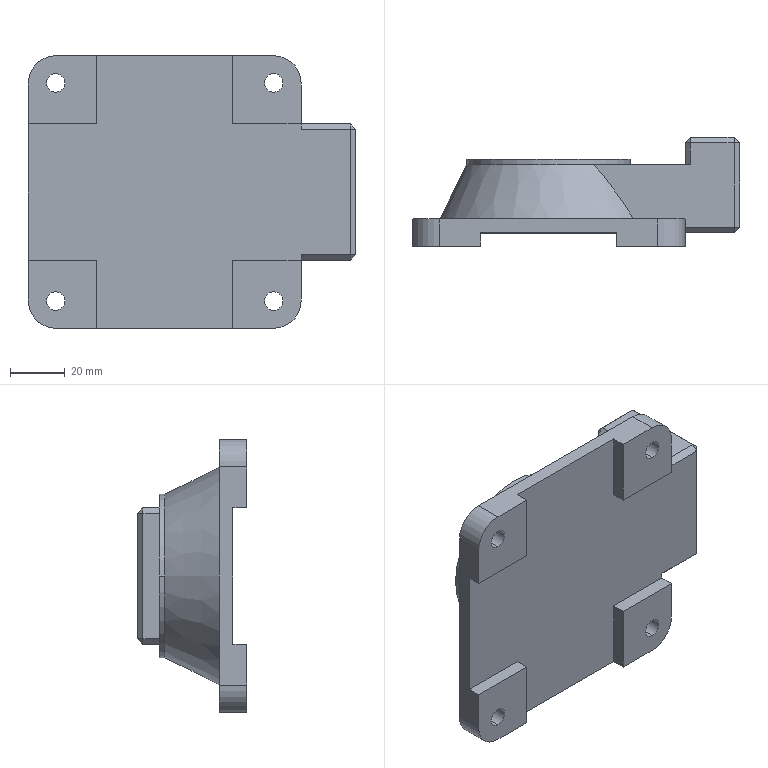Part | SolidWorks | features ICE 3, Cut 2, Chamfer 1, Extrusion 1, Fillet 1, HoleWzd 1, Revolution 1 | 1 solid | 58 faces | box 120 x 40 x 100 mm | volume 196028 mm3 | plane 43 | cylinder 14 | cone 1 | commonest cylinder face diameters 6.8 x8 20 x4 60 x2